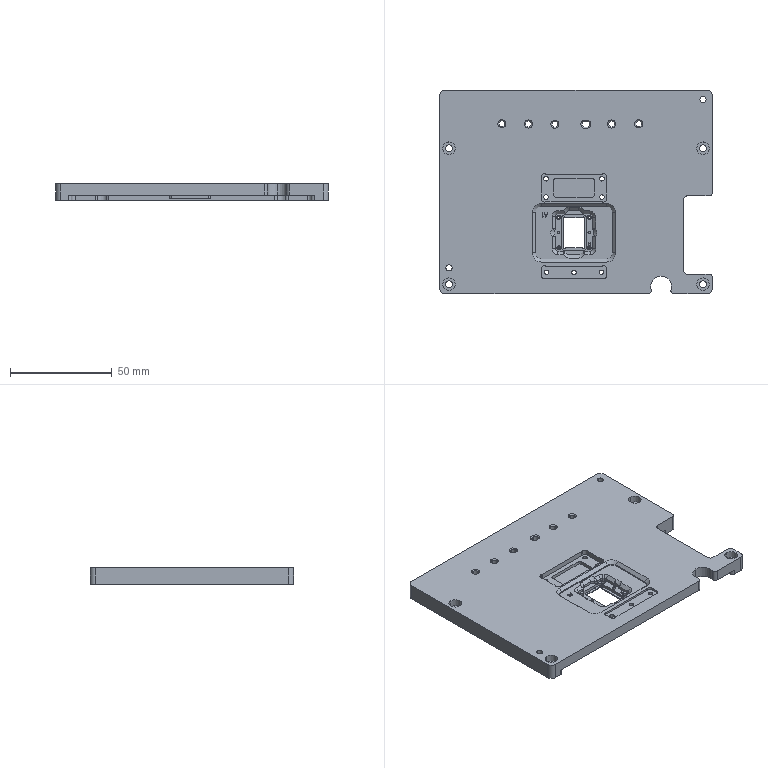NC program | NX | posted with a generic post | part box 134 x 100 x 8 mm
Lines 1537 to 2718 of 3418:
(ZLEVEL_PROFILE_COPY_COPY_COPY_1_COPY_COPY_1_COPY_COPY_COPY_1_COPY_COPY_1_COPY )
N3036 T20 M6
N3038 G54
N3040 G17 G0 G90 X2.531 Y-10.727 S9500 M3
N3042 G43 Z30. H20
N3044 Z0.1
N3046 G94 G1 X2.5 Y-10.6 Z0.093 F1000.
N3048 Y-8.627 Z-0.01
N3050 X2.387 Y-8.335 Z-0.027
N3052 X2.165 Y-8.113 Z-0.043
N3054 X1.873 Y-8. Z-0.06
N3056 X0.127 Z-0.151
N3058 X-0.165 Y-8.113 Z-0.167
N3060 X-0.387 Y-8.335 Z-0.184
N3062 X-0.5 Y-8.627 Z-0.2
N3064 Y-10.6 Z-0.304
N3066 X-0.629 Y-11.134 Z-0.333
N3068 X-0.898 Y-11.614 Z-0.361
N3070 X-1.286 Y-12.002 Z-0.39
N3072 X-1.766 Y-12.271 Z-0.419
N3074 X-2.3 Y-12.4 Z-0.448
N3076 X-4.337 Z-0.554
N3078 X-4.521 Y-12.501 Z-0.565
N3080 X-4.614 Y-12.649 Z-0.575
N3082 X-4.633 Y-12.814 Z-0.583
N3084 X-4.581 Y-12.971 Z-0.592
N3086 X-4.468 Y-13.093 Z-0.601
N3088 X-4.254 Y-13.176 Z-0.613
N3090 X-4.012 Y-13.366 Z-0.629
N3092 X-3.839 Y-13.62 Z-0.645
N3094 X-3.75 Y-13.914 Z-0.661
N3096 Y-20. Z-0.98
N3098 Y-25.944
N3100 G2 X-4.386 Y-26.876 R1.
N3102 G3 X-4.25 Y-27.6 R0.375
N3104 G1 X-2.5
N3106 G2 X-0.5 Y-29.6 R2.
N3108 G1 Y-31.25
N3110 G3 X0.25 Y-32. R0.75
N3112 G1 X1.75
N3114 G3 X2.5 Y-31.25 R0.75
N3116 G1 Y-29.6
N3118 G2 X4.5 Y-27.6 R2.
N3120 G1 X6.25
N3122 G3 X6.386 Y-26.876 R0.375
N3124 G2 X5.75 Y-25.944 R1.
N3126 G1 Y-14.056
N3128 G2 X6.386 Y-13.124 R1.
N3130 G3 X6.25 Y-12.4 R0.375
N3132 G1 X4.5
N3134 G2 X2.5 Y-10.4 R2.
N3136 G1 Y-8.75
N3138 G3 X1.75 Y-8. R0.75
N3140 G1 X0.25
N3142 G3 X-0.5 Y-8.75 R0.75
N3144 G1 Y-10.4
N3146 G2 X-2.5 Y-12.4 R2.
N3148 G1 X-4.25
N3150 G3 X-4.386 Y-13.124 R0.375
N3152 G2 X-3.75 Y-14.056 R1.
N3154 G1 Y-20.
N3156 Y-23.867 Z-1.048
N3158 Y-25.944
N3160 G2 X-4.386 Y-26.876 R1.
N3162 G3 X-4.25 Y-27.6 R0.375
N3164 G1 X-2.5
N3166 G2 X-0.5 Y-29.6 R2.
N3168 G1 Y-31.25
N3170 G3 X0.25 Y-32. R0.75
N3172 G1 X1.75
N3174 G3 X2.5 Y-31.25 R0.75
N3176 G1 Y-29.6
N3178 G2 X4.5 Y-27.6 R2.
N3180 G1 X6.25
N3182 G3 X6.386 Y-26.876 R0.375
N3184 G2 X5.75 Y-25.944 R1.
N3186 G1 Y-14.056
N3188 G2 X6.386 Y-13.124 R1.
N3190 G3 X6.25 Y-12.4 R0.375
N3192 G1 X4.5
N3194 G2 X2.5 Y-10.4 R2.
N3196 G1 Y-8.75
N3198 G3 X1.75 Y-8. R0.75
N3200 G1 X0.25
N3202 G3 X-0.5 Y-8.75 R0.75
N3204 G1 Y-10.4
N3206 G2 X-2.5 Y-12.4 R2.
N3208 G1 X-4.25
N3210 G3 X-4.386 Y-13.124 R0.375
N3212 G2 X-3.75 Y-14.056 R1.
N3214 G1 Y-20.
N3216 Y-23.867 Z-1.115
N3218 Y-25.944
N3220 G2 X-4.386 Y-26.876 R1.
N3222 G3 X-4.25 Y-27.6 R0.375
N3224 G1 X-2.5
N3226 G2 X-0.5 Y-29.6 R2.
N3228 G1 Y-31.25
N3230 G3 X0.25 Y-32. R0.75
N3232 G1 X1.75
N3234 G3 X2.5 Y-31.25 R0.75
N3236 G1 Y-29.6
N3238 G2 X4.5 Y-27.6 R2.
N3240 G1 X6.25
N3242 G3 X6.386 Y-26.876 R0.375
N3244 G2 X5.75 Y-25.944 R1.
N3246 G1 Y-14.056
N3248 G2 X6.386 Y-13.124 R1.
N3250 G3 X6.25 Y-12.4 R0.375
N3252 G1 X4.5
N3254 G2 X2.5 Y-10.4 R2.
N3256 G1 Y-8.75
N3258 G3 X1.75 Y-8. R0.75
N3260 G1 X0.25
N3262 G3 X-0.5 Y-8.75 R0.75
N3264 G1 Y-10.4
N3266 G2 X-2.5 Y-12.4 R2.
N3268 G1 X-4.25
N3270 G3 X-4.386 Y-13.124 R0.375
N3272 G2 X-3.75 Y-14.056 R1.
N3274 G1 Y-20.
N3276 Y-23.867 Z-1.183
N3278 Y-25.944
N3280 G2 X-4.386 Y-26.876 R1.
N3282 G3 X-4.25 Y-27.6 R0.375
N3284 G1 X-2.5
N3286 G2 X-0.5 Y-29.6 R2.
N3288 G1 Y-31.25
N3290 G3 X0.25 Y-32. R0.75
N3292 G1 X1.75
N3294 G3 X2.5 Y-31.25 R0.75
N3296 G1 Y-29.6
N3298 G2 X4.5 Y-27.6 R2.
N3300 G1 X6.25
N3302 G3 X6.386 Y-26.876 R0.375
N3304 G2 X5.75 Y-25.944 R1.
N3306 G1 Y-14.056
N3308 G2 X6.386 Y-13.124 R1.
N3310 G3 X6.25 Y-12.4 R0.375
N3312 G1 X4.5
N3314 G2 X2.5 Y-10.4 R2.
N3316 G1 Y-8.75
N3318 G3 X1.75 Y-8. R0.75
N3320 G1 X0.25
N3322 G3 X-0.5 Y-8.75 R0.75
N3324 G1 Y-10.4
N3326 G2 X-2.5 Y-12.4 R2.
N3328 G1 X-4.25
N3330 G3 X-4.386 Y-13.124 R0.375
N3332 G2 X-3.75 Y-14.056 R1.
N3334 G1 Y-20.
N3336 Y-23.867 Z-1.25
N3338 Y-25.944
N3340 G2 X-4.386 Y-26.876 R1.
N3342 G3 X-4.25 Y-27.6 R0.375
N3344 G1 X-2.5
N3346 G2 X-0.5 Y-29.6 R2.
N3348 G1 Y-31.25
N3350 G3 X0.25 Y-32. R0.75
N3352 G1 X1.75
N3354 G3 X2.5 Y-31.25 R0.75
N3356 G1 Y-29.6
N3358 G2 X4.5 Y-27.6 R2.
N3360 G1 X6.25
N3362 G3 X6.386 Y-26.876 R0.375
N3364 G2 X5.75 Y-25.944 R1.
N3366 G1 Y-14.056
N3368 G2 X6.386 Y-13.124 R1.
N3370 G3 X6.25 Y-12.4 R0.375
N3372 G1 X4.5
N3374 G2 X2.5 Y-10.4 R2.
N3376 G1 Y-8.75
N3378 G3 X1.75 Y-8. R0.75
N3380 G1 X0.25
N3382 G3 X-0.5 Y-8.75 R0.75
N3384 G1 Y-10.4
N3386 G2 X-2.5 Y-12.4 R2.
N3388 G1 X-4.25
N3390 G3 X-4.386 Y-13.124 R0.375
N3392 G2 X-3.75 Y-14.056 R1.
N3394 G1 Y-23.867
N3396 Z-0.25
N3398 G0 Z30.
(ZLEVEL_PROFILE_COPY_COPY_COPY_1_COPY_COPY_1_COPY_COPY_COPY_1_COPY_COPY_1_COPY_)
N3400 X0.084 Y-31.184
N3402 Z0.1
N3404 G1 X-0.086 Y-30.894 Z0.082
N3406 X-0.155 Y-30.482 Z0.06
N3408 X-0.073 Y-30.072 Z0.039
N3410 X0.076 Y-29.807 Z0.023
N3412 X0.292 Y-29.587 Z0.007
N3414 X0.559 Y-29.433 Z-0.01
N3416 X0.857 Y-29.354 Z-0.026
N3418 X1.161 Y-29.356 Z-0.042
N3420 X1.469 Y-29.445 Z-0.059
N3422 X1.742 Y-29.615 Z-0.075
N3424 X1.957 Y-29.853 Z-0.092
N3426 X2.092 Y-30.124 Z-0.108
N3428 X2.155 Y-30.524 Z-0.129
N3430 X2.075 Y-30.922 Z-0.151
N3432 X1.864 Y-31.267 Z-0.172
N3434 X1.546 Y-31.518 Z-0.193
N3436 X1.161 Y-31.644 Z-0.214
N3438 X1. Y-31.645 Z-0.223
N3440 X0.848 Z-0.231
N3442 X0.451 Y-31.516 Z-0.253
N3444 X0.125 Y-31.254 Z-0.274
N3446 X-0.086 Y-30.894 Z-0.296
N3448 X-0.155 Y-30.482 Z-0.318
N3450 X-0.073 Y-30.072 Z-0.34
N3452 X0.076 Y-29.807 Z-0.356
N3454 X0.292 Y-29.587 Z-0.372
N3456 X0.559 Y-29.433 Z-0.388
N3458 X0.857 Y-29.354 Z-0.405
N3460 X1.161 Y-29.356 Z-0.42
N3462 X1.469 Y-29.445 Z-0.437
N3464 X1.742 Y-29.615 Z-0.454
N3466 X1.957 Y-29.853 Z-0.471
N3468 X2.092 Y-30.124 Z-0.487
N3470 X2.155 Y-30.524 Z-0.508
N3472 X2.075 Y-30.922 Z-0.529
N3474 X1.864 Y-31.267 Z-0.55
N3476 X1.546 Y-31.518 Z-0.572
N3478 X1.161 Y-31.644 Z-0.593
N3480 X1. Y-31.645 Z-0.601
N3482 X0.848 Z-0.609
N3484 X0.451 Y-31.516 Z-0.631
N3486 X0.125 Y-31.254 Z-0.653
N3488 X-0.086 Y-30.894 Z-0.675
N3490 X-0.155 Y-30.482 Z-0.697
N3492 X-0.073 Y-30.072 Z-0.719
N3494 X0.076 Y-29.807 Z-0.735
N3496 X0.292 Y-29.587 Z-0.751
N3498 X0.559 Y-29.433 Z-0.767
N3500 X0.857 Y-29.354 Z-0.783
N3502 X1.161 Y-29.356 Z-0.799
N3504 X1.469 Y-29.445 Z-0.816
N3506 X1.742 Y-29.615 Z-0.833
N3508 X1.957 Y-29.853 Z-0.85
N3510 X2.092 Y-30.124 Z-0.865
N3512 X2.155 Y-30.524 Z-0.887
N3514 X2.075 Y-30.922 Z-0.908
N3516 X1.864 Y-31.267 Z-0.929
N3518 X1.546 Y-31.518 Z-0.95
N3520 X1.161 Y-31.644 Z-0.972
N3522 X1. Y-31.645 Z-0.98
N3524 G2 X-0.145 Y-30.5 R1.145
N3526 X1. Y-31.645 R-1.145
N3528 G1 X0.928 Y-31.643 Z-0.981
N3530 X0.857 Y-31.636 Z-0.983
N3532 X0.786 Y-31.625 Z-0.984
N3534 X0.717 Y-31.609 Z-0.985
N3536 X0.648 Y-31.589 Z-0.986
N3538 X0.58 Y-31.565 Z-0.988
N3540 X0.515 Y-31.537 Z-0.989
N3542 X0.451 Y-31.505 Z-0.99
N3544 X0.389 Y-31.468 Z-0.991
N3546 X0.33 Y-31.428 Z-0.993
N3548 X0.273 Y-31.385 Z-0.994
N3550 X0.219 Y-31.337 Z-0.995
N3552 X0.168 Y-31.287 Z-0.996
N3554 X0.121 Y-31.233 Z-0.998
N3556 X0.077 Y-31.177 Z-0.999
N3558 X0.036 Y-31.118 Z-1.
N3560 X-0.001 Y-31.057 Z-1.001
N3562 X-0.033 Y-30.993 Z-1.003
N3564 X-0.062 Y-30.927 Z-1.004
N3566 X-0.087 Y-30.86 Z-1.005
N3568 X-0.107 Y-30.791 Z-1.006
N3570 X-0.123 Y-30.722 Z-1.008
N3572 X-0.135 Y-30.651 Z-1.009
N3574 X-0.142 Y-30.58 Z-1.01
N3576 X-0.145 Y-30.508 Z-1.011
N3578 X-0.143 Y-30.437 Z-1.013
N3580 X-0.137 Y-30.365 Z-1.014
N3582 X-0.126 Y-30.295 Z-1.015
N3584 X-0.111 Y-30.225 Z-1.016
N3586 X-0.092 Y-30.156 Z-1.018
N3588 X-0.068 Y-30.088 Z-1.019
N3590 X-0.04 Y-30.022 Z-1.02
N3592 X-0.009 Y-29.958 Z-1.021
N3594 X0.027 Y-29.896 Z-1.023
N3596 X0.067 Y-29.836 Z-1.024
N3598 X0.11 Y-29.779 Z-1.025
N3600 X0.157 Y-29.725 Z-1.026
N3602 X0.207 Y-29.674 Z-1.028
N3604 X0.26 Y-29.626 Z-1.029
N3606 X0.316 Y-29.581 Z-1.03
N3608 X0.375 Y-29.541 Z-1.031
N3610 X0.436 Y-29.503 Z-1.033
N3612 X0.5 Y-29.47 Z-1.034
N3614 X0.565 Y-29.441 Z-1.035
N3616 X0.632 Y-29.416 Z-1.036
N3618 X0.701 Y-29.395 Z-1.038
N3620 X0.77 Y-29.378 Z-1.039
N3622 X0.841 Y-29.366 Z-1.04
N3624 X0.912 Y-29.358 Z-1.041
N3626 X0.984 Y-29.355 Z-1.043
N3628 X1.055 Y-29.356 Z-1.044
N3630 X1.126 Y-29.362 Z-1.045
N3632 X1.197 Y-29.372 Z-1.046
N3634 X1.267 Y-29.387 Z-1.048
N3636 X1.337 Y-29.406 Z-1.049
N3638 X1.404 Y-29.429 Z-1.05
N3640 X1.47 Y-29.456 Z-1.051
N3642 X1.535 Y-29.488 Z-1.053
N3644 X1.597 Y-29.523 Z-1.054
N3646 X1.657 Y-29.562 Z-1.055
N3648 X1.714 Y-29.605 Z-1.056
N3650 X1.769 Y-29.651 Z-1.058
N3652 X1.82 Y-29.701 Z-1.059
N3654 X1.869 Y-29.754 Z-1.06
N3656 G2 X1. Y-31.645 R1.145
N3658 G1 X0.928 Y-31.643 Z-1.061
N3660 X0.857 Y-31.636 Z-1.063
N3662 X0.786 Y-31.625 Z-1.064
N3664 X0.717 Y-31.609 Z-1.065
N3666 X0.648 Y-31.589 Z-1.066
N3668 X0.58 Y-31.565 Z-1.068
N3670 X0.515 Y-31.537 Z-1.069
N3672 X0.451 Y-31.505 Z-1.07
N3674 X0.389 Y-31.468 Z-1.071
N3676 X0.33 Y-31.428 Z-1.073
N3678 X0.273 Y-31.385 Z-1.074
N3680 X0.219 Y-31.337 Z-1.075
N3682 X0.168 Y-31.287 Z-1.076
N3684 X0.121 Y-31.233 Z-1.078
N3686 X0.077 Y-31.177 Z-1.079
N3688 X0.036 Y-31.118 Z-1.08
N3690 X-0.001 Y-31.057 Z-1.081
N3692 X-0.034 Y-30.993 Z-1.083
N3694 X-0.062 Y-30.927 Z-1.084
N3696 X-0.087 Y-30.86 Z-1.085
N3698 X-0.107 Y-30.791 Z-1.086
N3700 X-0.123 Y-30.722 Z-1.088
N3702 X-0.135 Y-30.651 Z-1.089
N3704 X-0.142 Y-30.58 Z-1.09
N3706 X-0.145 Y-30.508 Z-1.091
N3708 X-0.143 Y-30.437 Z-1.093
N3710 X-0.137 Y-30.365 Z-1.094
N3712 X-0.126 Y-30.295 Z-1.095
N3714 X-0.111 Y-30.225 Z-1.096
N3716 X-0.092 Y-30.156 Z-1.098
N3718 X-0.068 Y-30.088 Z-1.099
N3720 X-0.04 Y-30.022 Z-1.1
N3722 X-0.009 Y-29.958 Z-1.101
N3724 X0.027 Y-29.896 Z-1.103
N3726 X0.067 Y-29.836 Z-1.104
N3728 X0.11 Y-29.779 Z-1.105
N3730 X0.157 Y-29.725 Z-1.106
N3732 X0.207 Y-29.674 Z-1.108
N3734 X0.26 Y-29.626 Z-1.109
N3736 X0.316 Y-29.581 Z-1.11
N3738 X0.375 Y-29.541 Z-1.111
N3740 X0.436 Y-29.503 Z-1.113
N3742 X0.5 Y-29.47 Z-1.114
N3744 X0.565 Y-29.441 Z-1.115
N3746 X0.632 Y-29.416 Z-1.116
N3748 X0.701 Y-29.395 Z-1.118
N3750 X0.77 Y-29.378 Z-1.119
N3752 X0.841 Y-29.366 Z-1.12
N3754 X0.912 Y-29.358 Z-1.121
N3756 X0.984 Y-29.355 Z-1.123
N3758 X1.055 Y-29.356 Z-1.124
N3760 X1.126 Y-29.362 Z-1.125
N3762 X1.197 Y-29.372 Z-1.126
N3764 X1.268 Y-29.386 Z-1.128
N3766 X1.337 Y-29.406 Z-1.129
N3768 X1.404 Y-29.429 Z-1.13
N3770 X1.47 Y-29.456 Z-1.131
N3772 X1.535 Y-29.488 Z-1.133
N3774 G2 X1. Y-31.645 R1.145
N3776 G1 X0.928 Y-31.643 Z-1.134
N3778 X0.857 Y-31.636 Z-1.135
N3780 X0.786 Y-31.625 Z-1.136
N3782 X0.717 Y-31.609 Z-1.138
N3784 X0.648 Y-31.589 Z-1.139
N3786 X0.58 Y-31.565 Z-1.14
N3788 X0.515 Y-31.537 Z-1.141
N3790 X0.451 Y-31.505 Z-1.143
N3792 X0.389 Y-31.468 Z-1.144
N3794 X0.33 Y-31.428 Z-1.145
N3796 X0.273 Y-31.385 Z-1.146
N3798 X0.219 Y-31.337 Z-1.148
N3800 X0.168 Y-31.287 Z-1.149
N3802 X0.121 Y-31.233 Z-1.15
N3804 X0.077 Y-31.177 Z-1.151
N3806 X0.036 Y-31.118 Z-1.153
N3808 X-0.001 Y-31.057 Z-1.154
N3810 X-0.033 Y-30.993 Z-1.155
N3812 X-0.062 Y-30.927 Z-1.156
N3814 X-0.087 Y-30.86 Z-1.158
N3816 X-0.107 Y-30.791 Z-1.159
N3818 X-0.123 Y-30.722 Z-1.16
N3820 X-0.135 Y-30.651 Z-1.161
N3822 X-0.142 Y-30.58 Z-1.163
N3824 X-0.145 Y-30.508 Z-1.164
N3826 X-0.143 Y-30.437 Z-1.165
N3828 X-0.137 Y-30.365 Z-1.166
N3830 X-0.126 Y-30.295 Z-1.168
N3832 X-0.111 Y-30.225 Z-1.169
N3834 X-0.092 Y-30.156 Z-1.17
N3836 X-0.068 Y-30.088 Z-1.171
N3838 X-0.04 Y-30.022 Z-1.173
N3840 X-0.009 Y-29.958 Z-1.174
N3842 X0.027 Y-29.896 Z-1.175
N3844 X0.067 Y-29.836 Z-1.176
N3846 X0.11 Y-29.779 Z-1.178
N3848 X0.157 Y-29.725 Z-1.179
N3850 X0.207 Y-29.674 Z-1.18
N3852 X0.26 Y-29.626 Z-1.181
N3854 X0.316 Y-29.581 Z-1.183
N3856 X0.375 Y-29.541 Z-1.184
N3858 X0.436 Y-29.503 Z-1.185
N3860 X0.5 Y-29.47 Z-1.186
N3862 X0.565 Y-29.441 Z-1.188
N3864 X0.632 Y-29.416 Z-1.189
N3866 X0.7 Y-29.395 Z-1.19
N3868 X0.77 Y-29.378 Z-1.191
N3870 X0.841 Y-29.366 Z-1.193
N3872 X0.912 Y-29.358 Z-1.194
N3874 X0.984 Y-29.355 Z-1.195
N3876 X1.055 Y-29.356 Z-1.196
N3878 X1.126 Y-29.362 Z-1.198
N3880 X1.197 Y-29.372 Z-1.199
N3882 X1.267 Y-29.387 Z-1.2
N3884 X1.337 Y-29.406 Z-1.201
N3886 X1.404 Y-29.428 Z-1.203
N3888 X1.47 Y-29.456 Z-1.204
N3890 X1.535 Y-29.488 Z-1.205
N3892 G2 X1. Y-31.645 R1.145
N3894 G1 X0.928 Y-31.643 Z-1.206
N3896 X0.857 Y-31.636 Z-1.208
N3898 X0.786 Y-31.625 Z-1.209
N3900 X0.717 Y-31.609 Z-1.21
N3902 X0.648 Y-31.589 Z-1.211
N3904 X0.58 Y-31.565 Z-1.213
N3906 X0.515 Y-31.537 Z-1.214
N3908 X0.451 Y-31.505 Z-1.215
N3910 X0.389 Y-31.468 Z-1.216
N3912 X0.329 Y-31.429 Z-1.218
N3914 X0.273 Y-31.385 Z-1.219
N3916 X0.219 Y-31.337 Z-1.22
N3918 X0.168 Y-31.287 Z-1.221
N3920 X0.121 Y-31.233 Z-1.223
N3922 X0.077 Y-31.177 Z-1.224
N3924 X0.036 Y-31.118 Z-1.225
N3926 X-0.001 Y-31.057 Z-1.226
N3928 X-0.033 Y-30.993 Z-1.228
N3930 X-0.062 Y-30.927 Z-1.229
N3932 X-0.087 Y-30.86 Z-1.23
N3934 X-0.107 Y-30.791 Z-1.231
N3936 X-0.123 Y-30.722 Z-1.233
N3938 X-0.135 Y-30.651 Z-1.234
N3940 X-0.142 Y-30.58 Z-1.235
N3942 X-0.145 Y-30.508 Z-1.236
N3944 X-0.143 Y-30.437 Z-1.238
N3946 X-0.137 Y-30.365 Z-1.239
N3948 X-0.126 Y-30.295 Z-1.24
N3950 X-0.111 Y-30.225 Z-1.241
N3952 X-0.092 Y-30.156 Z-1.243
N3954 X-0.068 Y-30.088 Z-1.244
N3956 X-0.04 Y-30.022 Z-1.245
N3958 X-0.009 Y-29.958 Z-1.246
N3960 X0.027 Y-29.896 Z-1.248
N3962 X0.067 Y-29.836 Z-1.249
N3964 X0.11 Y-29.779 Z-1.25
N3966 X0.157 Y-29.725 Z-1.251
N3968 X0.207 Y-29.674 Z-1.253
N3970 X0.26 Y-29.626 Z-1.254
N3972 X0.316 Y-29.581 Z-1.255
N3974 X0.375 Y-29.541 Z-1.256
N3976 X0.436 Y-29.503 Z-1.258
N3978 X0.5 Y-29.47 Z-1.259
N3980 X0.565 Y-29.441 Z-1.26
N3982 X0.632 Y-29.416 Z-1.261
N3984 X0.7 Y-29.394 Z-1.263
N3986 X0.77 Y-29.378 Z-1.264
N3988 X0.841 Y-29.366 Z-1.265
N3990 X0.912 Y-29.358 Z-1.266
N3992 X0.984 Y-29.355 Z-1.268
N3994 X1.055 Y-29.356 Z-1.269
N3996 X1.126 Y-29.362 Z-1.27
N3998 X1.197 Y-29.372 Z-1.271
N4000 X1.267 Y-29.387 Z-1.273
N4002 X1.337 Y-29.406 Z-1.274
N4004 X1.404 Y-29.428 Z-1.275
N4006 X1.47 Y-29.456 Z-1.276
N4008 X1.535 Y-29.488 Z-1.278
N4010 G2 X1. Y-31.645 R1.145
N4012 G1 X0.928 Y-31.643 Z-1.279
N4014 X0.857 Y-31.636 Z-1.28
N4016 X0.786 Y-31.625 Z-1.281
N4018 X0.717 Y-31.609 Z-1.283
N4020 X0.648 Y-31.589 Z-1.284
N4022 X0.58 Y-31.566 Z-1.285
N4024 X0.515 Y-31.537 Z-1.286
N4026 X0.451 Y-31.505 Z-1.288
N4028 X0.389 Y-31.468 Z-1.289
N4030 X0.33 Y-31.428 Z-1.29
N4032 X0.273 Y-31.385 Z-1.291
N4034 X0.219 Y-31.337 Z-1.293
N4036 X0.168 Y-31.287 Z-1.294
N4038 X0.121 Y-31.233 Z-1.295
N4040 X0.077 Y-31.177 Z-1.296
N4042 X0.036 Y-31.118 Z-1.298
N4044 X-0.001 Y-31.057 Z-1.299
N4046 X-0.034 Y-30.993 Z-1.3
N4048 X-0.062 Y-30.927 Z-1.301
N4050 X-0.087 Y-30.86 Z-1.303
N4052 X-0.107 Y-30.791 Z-1.304
N4054 X-0.123 Y-30.722 Z-1.305
N4056 X-0.135 Y-30.651 Z-1.306
N4058 X-0.142 Y-30.58 Z-1.308
N4060 X-0.145 Y-30.508 Z-1.309
N4062 X-0.143 Y-30.437 Z-1.31
N4064 X-0.137 Y-30.365 Z-1.311
N4066 X-0.126 Y-30.295 Z-1.313
N4068 X-0.111 Y-30.225 Z-1.314
N4070 X-0.092 Y-30.156 Z-1.315
N4072 X-0.068 Y-30.088 Z-1.316
N4074 X-0.04 Y-30.022 Z-1.318
N4076 X-0.009 Y-29.958 Z-1.319
N4078 X0.027 Y-29.896 Z-1.32
N4080 X0.067 Y-29.836 Z-1.321
N4082 X0.11 Y-29.779 Z-1.323
N4084 X0.157 Y-29.725 Z-1.324
N4086 X0.207 Y-29.674 Z-1.325
N4088 X0.26 Y-29.626 Z-1.326
N4090 X0.316 Y-29.581 Z-1.328
N4092 X0.375 Y-29.541 Z-1.329
N4094 X0.436 Y-29.503 Z-1.33
N4096 X0.5 Y-29.47 Z-1.331
N4098 X0.565 Y-29.441 Z-1.333
N4100 X0.632 Y-29.416 Z-1.334
N4102 X0.701 Y-29.395 Z-1.335
N4104 X0.77 Y-29.378 Z-1.336
N4106 X0.841 Y-29.366 Z-1.338
N4108 X0.912 Y-29.358 Z-1.339
N4110 X0.984 Y-29.355 Z-1.34
N4112 X1.055 Y-29.356 Z-1.341
N4114 X1.127 Y-29.361 Z-1.343
N4116 X1.197 Y-29.372 Z-1.344
N4118 X1.268 Y-29.386 Z-1.345
N4120 X1.337 Y-29.406 Z-1.346
N4122 X1.404 Y-29.428 Z-1.348
N4124 X1.47 Y-29.456 Z-1.349
N4126 X1.535 Y-29.488 Z-1.35
N4128 G2 X2.012 Y-31.035 R1.145
N4130 X1.535 Y-29.488 R-1.145
N4132 G1 Z-0.35
N4134 G0 Z30.
N4136 X0.084 Y-10.184
N4138 Z0.1
N4140 G1 X-0.086 Y-9.894 Z0.082
N4142 X-0.155 Y-9.482 Z0.06
N4144 X-0.073 Y-9.072 Z0.039
N4146 X0.076 Y-8.807 Z0.023
N4148 X0.292 Y-8.587 Z0.007
N4150 X0.559 Y-8.433 Z-0.01
N4152 X0.857 Y-8.354 Z-0.026
N4154 X1.161 Y-8.356 Z-0.042
N4156 X1.469 Y-8.445 Z-0.059
N4158 X1.742 Y-8.615 Z-0.075
N4160 X1.957 Y-8.853 Z-0.092
N4162 X2.092 Y-9.124 Z-0.108
N4164 X2.155 Y-9.524 Z-0.129
N4166 X2.075 Y-9.922 Z-0.151
N4168 X1.864 Y-10.267 Z-0.172
N4170 X1.546 Y-10.518 Z-0.193
N4172 X1.161 Y-10.644 Z-0.214
N4174 X1. Y-10.645 Z-0.223
N4176 X0.848 Z-0.231
N4178 X0.451 Y-10.516 Z-0.253
N4180 X0.125 Y-10.254 Z-0.274
N4182 X-0.086 Y-9.894 Z-0.296
N4184 X-0.155 Y-9.482 Z-0.318
N4186 X-0.073 Y-9.072 Z-0.34
N4188 X0.076 Y-8.807 Z-0.356
N4190 X0.292 Y-8.587 Z-0.372
N4192 X0.559 Y-8.433 Z-0.388
N4194 X0.857 Y-8.354 Z-0.405
N4196 X1.161 Y-8.356 Z-0.42
N4198 X1.469 Y-8.445 Z-0.437
N4200 X1.742 Y-8.615 Z-0.454
N4202 X1.957 Y-8.853 Z-0.471
N4204 X2.092 Y-9.124 Z-0.487
N4206 X2.155 Y-9.524 Z-0.508
N4208 X2.075 Y-9.922 Z-0.529
N4210 X1.864 Y-10.267 Z-0.55
N4212 X1.546 Y-10.518 Z-0.572
N4214 X1.161 Y-10.644 Z-0.593
N4216 X1. Y-10.645 Z-0.601
N4218 X0.848 Z-0.609
N4220 X0.451 Y-10.516 Z-0.631
N4222 X0.125 Y-10.254 Z-0.653
N4224 X-0.086 Y-9.894 Z-0.675
N4226 X-0.155 Y-9.482 Z-0.697
N4228 X-0.073 Y-9.072 Z-0.719
N4230 X0.076 Y-8.807 Z-0.735
N4232 X0.292 Y-8.587 Z-0.751
N4234 X0.559 Y-8.433 Z-0.767
N4236 X0.857 Y-8.354 Z-0.783
N4238 X1.161 Y-8.356 Z-0.799
N4240 X1.469 Y-8.445 Z-0.816
N4242 X1.742 Y-8.615 Z-0.833
N4244 X1.957 Y-8.853 Z-0.85
N4246 X2.092 Y-9.124 Z-0.865
N4248 X2.155 Y-9.524 Z-0.887
N4250 X2.075 Y-9.922 Z-0.908
N4252 X1.864 Y-10.267 Z-0.929
N4254 X1.546 Y-10.518 Z-0.95
N4256 X1.161 Y-10.644 Z-0.972
N4258 X1. Y-10.645 Z-0.98
N4260 G2 X-0.145 Y-9.5 R1.145
N4262 X1. Y-10.645 R-1.145
N4264 G1 X0.928 Y-10.643 Z-0.981
N4266 X0.857 Y-10.636 Z-0.983
N4268 X0.786 Y-10.625 Z-0.984
N4270 X0.717 Y-10.609 Z-0.985
N4272 X0.648 Y-10.589 Z-0.986
N4274 X0.58 Y-10.565 Z-0.988
N4276 X0.515 Y-10.537 Z-0.989
N4278 X0.451 Y-10.505 Z-0.99
N4280 X0.389 Y-10.468 Z-0.991
N4282 X0.33 Y-10.428 Z-0.993
N4284 X0.273 Y-10.385 Z-0.994
N4286 X0.219 Y-10.337 Z-0.995
N4288 X0.168 Y-10.287 Z-0.996
N4290 X0.121 Y-10.233 Z-0.998
N4292 X0.077 Y-10.177 Z-0.999
N4294 X0.036 Y-10.118 Z-1.
N4296 X-0.001 Y-10.057 Z-1.001
N4298 X-0.033 Y-9.993 Z-1.003
N4300 X-0.062 Y-9.927 Z-1.004
N4302 X-0.087 Y-9.86 Z-1.005
N4304 X-0.107 Y-9.791 Z-1.006
N4306 X-0.123 Y-9.722 Z-1.008
N4308 X-0.135 Y-9.651 Z-1.009
N4310 X-0.142 Y-9.58 Z-1.01
N4312 X-0.145 Y-9.508 Z-1.011
N4314 X-0.143 Y-9.437 Z-1.013
N4316 X-0.137 Y-9.365 Z-1.014
N4318 X-0.127 Y-9.295 Z-1.015
N4320 X-0.111 Y-9.225 Z-1.016
N4322 X-0.092 Y-9.156 Z-1.018
N4324 X-0.068 Y-9.088 Z-1.019
N4326 X-0.04 Y-9.022 Z-1.02
N4328 X-0.009 Y-8.958 Z-1.021
N4330 X0.027 Y-8.896 Z-1.023
N4332 X0.067 Y-8.836 Z-1.024
N4334 X0.11 Y-8.779 Z-1.025
N4336 X0.157 Y-8.725 Z-1.026
N4338 X0.207 Y-8.674 Z-1.028
N4340 X0.26 Y-8.626 Z-1.029
N4342 X0.316 Y-8.581 Z-1.03
N4344 X0.375 Y-8.541 Z-1.031
N4346 X0.436 Y-8.503 Z-1.033
N4348 X0.5 Y-8.47 Z-1.034
N4350 X0.565 Y-8.441 Z-1.035
N4352 X0.632 Y-8.416 Z-1.036
N4354 X0.701 Y-8.395 Z-1.038
N4356 X0.77 Y-8.378 Z-1.039
N4358 X0.841 Y-8.366 Z-1.04
N4360 X0.912 Y-8.358 Z-1.041
N4362 X0.984 Y-8.355 Z-1.043
N4364 X1.055 Y-8.356 Z-1.044
N4366 X1.126 Y-8.362 Z-1.045
N4368 X1.197 Y-8.372 Z-1.046
N4370 X1.267 Y-8.387 Z-1.048
N4372 X1.337 Y-8.406 Z-1.049
N4374 X1.404 Y-8.429 Z-1.05
N4376 X1.47 Y-8.456 Z-1.051
N4378 X1.535 Y-8.488 Z-1.053
N4380 X1.597 Y-8.523 Z-1.054
N4382 X1.657 Y-8.562 Z-1.055
N4384 X1.714 Y-8.605 Z-1.056
N4386 X1.769 Y-8.651 Z-1.058
N4388 X1.82 Y-8.701 Z-1.059
N4390 X1.869 Y-8.754 Z-1.06
N4392 G2 X1. Y-10.645 R1.145
N4394 G1 X0.928 Y-10.643 Z-1.061
N4396 X0.857 Y-10.636 Z-1.063
N4398 X0.786 Y-10.625 Z-1.064
N4400 X0.717 Y-10.609 Z-1.065
N4402 X0.648 Y-10.589 Z-1.066
N4404 X0.58 Y-10.565 Z-1.068
N4406 X0.515 Y-10.537 Z-1.069
N4408 X0.451 Y-10.505 Z-1.07
N4410 X0.389 Y-10.468 Z-1.071
N4412 X0.33 Y-10.428 Z-1.073
N4414 X0.273 Y-10.385 Z-1.074
N4416 X0.219 Y-10.337 Z-1.075
N4418 X0.168 Y-10.287 Z-1.076
N4420 X0.121 Y-10.233 Z-1.078
N4422 X0.077 Y-10.177 Z-1.079
N4424 X0.036 Y-10.118 Z-1.08
N4426 X-0.001 Y-10.057 Z-1.081
N4428 X-0.034 Y-9.993 Z-1.083
N4430 X-0.062 Y-9.927 Z-1.084
N4432 X-0.087 Y-9.86 Z-1.085
N4434 X-0.107 Y-9.791 Z-1.086
N4436 X-0.124 Y-9.722 Z-1.088
N4438 X-0.135 Y-9.651 Z-1.089
N4440 X-0.142 Y-9.58 Z-1.09
N4442 X-0.145 Y-9.508 Z-1.091
N4444 X-0.143 Y-9.437 Z-1.093
N4446 X-0.137 Y-9.365 Z-1.094
N4448 X-0.126 Y-9.295 Z-1.095
N4450 X-0.111 Y-9.225 Z-1.096
N4452 X-0.092 Y-9.156 Z-1.098
N4454 X-0.068 Y-9.088 Z-1.099
N4456 X-0.04 Y-9.022 Z-1.1
N4458 X-0.009 Y-8.958 Z-1.101
N4460 X0.027 Y-8.896 Z-1.103
N4462 X0.067 Y-8.836 Z-1.104
N4464 X0.11 Y-8.779 Z-1.105
N4466 X0.157 Y-8.725 Z-1.106
N4468 X0.207 Y-8.674 Z-1.108
N4470 X0.26 Y-8.626 Z-1.109
N4472 X0.316 Y-8.581 Z-1.11
N4474 X0.375 Y-8.541 Z-1.111
N4476 X0.436 Y-8.503 Z-1.113
N4478 X0.5 Y-8.47 Z-1.114
N4480 X0.565 Y-8.441 Z-1.115
N4482 X0.632 Y-8.416 Z-1.116
N4484 X0.701 Y-8.395 Z-1.118
N4486 X0.77 Y-8.378 Z-1.119
N4488 X0.841 Y-8.366 Z-1.12
N4490 X0.912 Y-8.358 Z-1.121
N4492 X0.984 Y-8.355 Z-1.123
N4494 X1.055 Y-8.356 Z-1.124
N4496 X1.126 Y-8.362 Z-1.125
N4498 X1.197 Y-8.372 Z-1.126
N4500 X1.267 Y-8.387 Z-1.128
N4502 X1.337 Y-8.406 Z-1.129
N4504 X1.404 Y-8.429 Z-1.13
N4506 X1.47 Y-8.456 Z-1.131
N4508 X1.535 Y-8.488 Z-1.133
N4510 G2 X1. Y-10.645 R1.145
N4512 G1 X0.928 Y-10.643 Z-1.134
N4514 X0.857 Y-10.636 Z-1.135
N4516 X0.786 Y-10.625 Z-1.136
N4518 X0.716 Y-10.61 Z-1.138
N4520 X0.648 Y-10.589 Z-1.139
N4522 X0.58 Y-10.566 Z-1.14
N4524 X0.515 Y-10.537 Z-1.141
N4526 X0.451 Y-10.505 Z-1.143
N4528 X0.389 Y-10.468 Z-1.144
N4530 X0.33 Y-10.428 Z-1.145
N4532 X0.273 Y-10.385 Z-1.146
N4534 X0.219 Y-10.338 Z-1.148
N4536 X0.168 Y-10.287 Z-1.149
N4538 X0.121 Y-10.233 Z-1.15
N4540 X0.077 Y-10.177 Z-1.151
N4542 X0.036 Y-10.118 Z-1.153
N4544 X-0.001 Y-10.057 Z-1.154
N4546 X-0.033 Y-9.993 Z-1.155
N4548 X-0.062 Y-9.927 Z-1.156
N4550 X-0.087 Y-9.86 Z-1.158
N4552 X-0.107 Y-9.791 Z-1.159
N4554 X-0.124 Y-9.722 Z-1.16
N4556 X-0.135 Y-9.651 Z-1.161
N4558 X-0.143 Y-9.58 Z-1.163
N4560 X-0.145 Y-9.508 Z-1.164
N4562 X-0.144 Y-9.437 Z-1.165
N4564 X-0.137 Y-9.365 Z-1.166
N4566 X-0.126 Y-9.295 Z-1.168
N4568 X-0.111 Y-9.225 Z-1.169
N4570 X-0.092 Y-9.156 Z-1.17
N4572 X-0.068 Y-9.088 Z-1.171
N4574 X-0.04 Y-9.022 Z-1.173
N4576 X-0.009 Y-8.958 Z-1.174
N4578 X0.027 Y-8.896 Z-1.175
N4580 X0.067 Y-8.836 Z-1.176
N4582 X0.11 Y-8.779 Z-1.178
N4584 X0.157 Y-8.725 Z-1.179
N4586 X0.207 Y-8.674 Z-1.18
N4588 X0.26 Y-8.626 Z-1.181
N4590 X0.316 Y-8.581 Z-1.183
N4592 X0.375 Y-8.541 Z-1.184
N4594 X0.436 Y-8.503 Z-1.185
N4596 X0.5 Y-8.47 Z-1.186
N4598 X0.565 Y-8.441 Z-1.188
N4600 X0.632 Y-8.416 Z-1.189
N4602 X0.7 Y-8.395 Z-1.19
N4604 X0.77 Y-8.378 Z-1.191
N4606 X0.841 Y-8.366 Z-1.193
N4608 X0.912 Y-8.358 Z-1.194
N4610 X0.984 Y-8.355 Z-1.195
N4612 X1.055 Y-8.356 Z-1.196
N4614 X1.126 Y-8.362 Z-1.198
N4616 X1.197 Y-8.372 Z-1.199
N4618 X1.267 Y-8.387 Z-1.2
N4620 X1.337 Y-8.406 Z-1.201
N4622 X1.404 Y-8.429 Z-1.203
N4624 X1.47 Y-8.456 Z-1.204
N4626 X1.535 Y-8.488 Z-1.205
N4628 G2 X1. Y-10.645 R1.145
N4630 G1 X0.928 Y-10.643 Z-1.206
N4632 X0.857 Y-10.636 Z-1.208
N4634 X0.786 Y-10.625 Z-1.209
N4636 X0.716 Y-10.61 Z-1.21
N4638 X0.648 Y-10.589 Z-1.211
N4640 X0.58 Y-10.566 Z-1.213
N4642 X0.515 Y-10.537 Z-1.214
N4644 X0.451 Y-10.505 Z-1.215
N4646 X0.389 Y-10.468 Z-1.216
N4648 X0.33 Y-10.428 Z-1.218
N4650 X0.273 Y-10.385 Z-1.219
N4652 X0.219 Y-10.338 Z-1.22
N4654 X0.168 Y-10.287 Z-1.221
N4656 X0.121 Y-10.233 Z-1.223
N4658 X0.077 Y-10.177 Z-1.224
N4660 X0.036 Y-10.118 Z-1.225
N4662 X-0.001 Y-10.057 Z-1.226
N4664 X-0.033 Y-9.993 Z-1.228
N4666 X-0.062 Y-9.927 Z-1.229
N4668 X-0.087 Y-9.86 Z-1.23
N4670 X-0.107 Y-9.791 Z-1.231
N4672 X-0.124 Y-9.722 Z-1.233
N4674 X-0.135 Y-9.651 Z-1.234
N4676 X-0.143 Y-9.58 Z-1.235
N4678 X-0.145 Y-9.508 Z-1.236
N4680 X-0.144 Y-9.437 Z-1.238
N4682 X-0.137 Y-9.365 Z-1.239
N4684 X-0.126 Y-9.295 Z-1.24
N4686 X-0.111 Y-9.225 Z-1.241
N4688 X-0.092 Y-9.156 Z-1.243
N4690 X-0.068 Y-9.088 Z-1.244
N4692 X-0.04 Y-9.022 Z-1.245
N4694 X-0.009 Y-8.958 Z-1.246
N4696 X0.027 Y-8.896 Z-1.248
N4698 X0.067 Y-8.836 Z-1.249
N4700 X0.11 Y-8.779 Z-1.25
N4702 X0.157 Y-8.725 Z-1.251
N4704 X0.207 Y-8.674 Z-1.253
N4706 X0.26 Y-8.626 Z-1.254
N4708 X0.316 Y-8.581 Z-1.255
N4710 X0.375 Y-8.541 Z-1.256
N4712 X0.436 Y-8.503 Z-1.258
N4714 X0.5 Y-8.47 Z-1.259
N4716 X0.565 Y-8.441 Z-1.26
N4718 X0.632 Y-8.416 Z-1.261
N4720 X0.7 Y-8.394 Z-1.263
N4722 X0.77 Y-8.378 Z-1.264
N4724 X0.841 Y-8.366 Z-1.265
N4726 X0.912 Y-8.358 Z-1.266
N4728 X0.984 Y-8.355 Z-1.268
N4730 X1.055 Y-8.356 Z-1.269
N4732 X1.126 Y-8.362 Z-1.27
N4734 X1.197 Y-8.372 Z-1.271
N4736 X1.267 Y-8.387 Z-1.273
N4738 X1.337 Y-8.406 Z-1.274
N4740 X1.404 Y-8.429 Z-1.275
N4742 X1.47 Y-8.456 Z-1.276
N4744 X1.535 Y-8.488 Z-1.278
N4746 G2 X1. Y-10.645 R1.145
N4748 G1 X0.928 Y-10.643 Z-1.279
N4750 X0.857 Y-10.636 Z-1.28
N4752 X0.786 Y-10.625 Z-1.281
N4754 X0.717 Y-10.609 Z-1.283
N4756 X0.648 Y-10.589 Z-1.284
N4758 X0.58 Y-10.566 Z-1.285
N4760 X0.515 Y-10.537 Z-1.286
N4762 X0.451 Y-10.505 Z-1.288
N4764 X0.389 Y-10.468 Z-1.289
N4766 X0.33 Y-10.428 Z-1.29
N4768 X0.273 Y-10.385 Z-1.291
N4770 X0.219 Y-10.337 Z-1.293
N4772 X0.168 Y-10.287 Z-1.294
N4774 X0.121 Y-10.233 Z-1.295
N4776 X0.077 Y-10.177 Z-1.296
N4778 X0.036 Y-10.118 Z-1.298
N4780 X-0.001 Y-10.057 Z-1.299
N4782 X-0.034 Y-9.993 Z-1.3
N4784 X-0.062 Y-9.927 Z-1.301
N4786 X-0.087 Y-9.86 Z-1.303
N4788 X-0.107 Y-9.791 Z-1.304
N4790 X-0.124 Y-9.722 Z-1.305
N4792 X-0.135 Y-9.651 Z-1.306
N4794 X-0.142 Y-9.58 Z-1.308
N4796 X-0.145 Y-9.508 Z-1.309
N4798 X-0.144 Y-9.437 Z-1.31
N4800 X-0.137 Y-9.365 Z-1.311
N4802 X-0.126 Y-9.295 Z-1.313
N4804 X-0.111 Y-9.225 Z-1.314
N4806 X-0.092 Y-9.156 Z-1.315
N4808 X-0.068 Y-9.088 Z-1.316
N4810 X-0.04 Y-9.022 Z-1.318
N4812 X-0.009 Y-8.958 Z-1.319
N4814 X0.027 Y-8.896 Z-1.32
N4816 X0.067 Y-8.836 Z-1.321
N4818 X0.11 Y-8.779 Z-1.323
N4820 X0.157 Y-8.725 Z-1.324
N4822 X0.207 Y-8.674 Z-1.325
N4824 X0.26 Y-8.626 Z-1.326
N4826 X0.316 Y-8.581 Z-1.328
N4828 X0.375 Y-8.541 Z-1.329
N4830 X0.436 Y-8.503 Z-1.33
N4832 X0.5 Y-8.47 Z-1.331
N4834 X0.565 Y-8.44 Z-1.333
N4836 X0.632 Y-8.416 Z-1.334
N4838 X0.701 Y-8.395 Z-1.335
N4840 X0.77 Y-8.378 Z-1.336
N4842 X0.841 Y-8.366 Z-1.338
N4844 X0.912 Y-8.358 Z-1.339
N4846 X0.984 Y-8.355 Z-1.34
N4848 X1.055 Y-8.356 Z-1.341
N4850 X1.126 Y-8.362 Z-1.343
N4852 X1.197 Y-8.372 Z-1.344
N4854 X1.267 Y-8.387 Z-1.345
N4856 X1.337 Y-8.406 Z-1.346
N4858 X1.404 Y-8.429 Z-1.348
N4860 X1.47 Y-8.456 Z-1.349
N4862 X1.535 Y-8.488 Z-1.35
N4864 G2 X2.012 Y-10.035 R1.145
N4866 X1.535 Y-8.488 R-1.145
N4868 G1 Z-0.35
N4870 G0 Z30.
N4872 M5
(11_COPY , TOOL : D6A45)
N4874 T01 M6
N4876 G54
N4878 G17 G0 G90 X-63.551 Y45.5 S9500 M3
N4880 G43 Z30. H1
N4882 Z3.
N4884 G94 G1 Z-1. F1000.
N4886 G3 X-62.5 Y44.449 R1.051
N4888 X-63.551 Y45.5 R-1.051
N4890 X-63.251 Y44.98 R0.6
N4892 G1 Z2.
N4894 G0 Z30.
N4896 X63.551 Y-37.296
N4898 Z3.
N4900 G1 Z-1.
N4902 G3 X62.5 Y-36.245 R1.051
N4904 X63.551 Y-37.296 R-1.051
N4906 X63.251 Y-36.777 R0.6
N4908 G1 Z2.
N4910 G0 Z30.
N4912 X63.291 Y21.5
N4914 Z3.
N4916 G1 Z-1.
N4918 G3 X62.5 Y22.291 R0.791
N4920 X63.291 Y21.5 R-0.791
N4922 X62.991 Y22.02 R0.6
N4924 G1 Z2.
N4926 G0 Z30.
N4928 X-63.291 Y21.5
N4930 Z3.
N4932 G1 Z-1.
N4934 G3 X-62.5 Y20.709 R0.791
N4936 X-63.291 Y21.5 R-0.791
N4938 X-62.991 Y20.98 R0.6
N4940 G1 Z2.
N4942 G0 Z30.
N4944 X63.291 Y-45.396
N4946 Z3.
N4948 G1 Z-1.
N4950 G3 X62.5 Y-44.605 R0.791
N4952 X63.291 Y-45.396 R-0.791
N4954 X62.991 Y-44.877 R0.6
N4956 G1 Z2.
N4958 G0 Z30.
N4960 X-63.291 Y-45.396
N4962 Z3.
N4964 G1 Z-1.
N4966 G3 X-62.5 Y-46.188 R0.791
N4968 X-63.291 Y-45.396 R-0.791
N4970 X-62.991 Y-45.916 R0.6
N4972 G1 Z2.
N4974 G0 Z30.
N4976 X-69.055 Y-48.479
N4978 Z2.
N4980 G1 Z-1.
N4982 X-68.259 Y-48.02
N4984 G3 X-67.959 Y-47.5 R0.6
N4986 G1 Y-41.964
N4988 G2 X-65.5 Y-39.506 R2.459
N4990 G1 X-60.219
N4992 G2 X-57.76 Y-41.964 R2.459
N4994 G1 Y-48.5
N4996 G2 X-60.219 Y-50.959 R2.459
N4998 G1 X-64.5
N5000 G2 X-67.959 Y-47.5 R3.459
N5002 G3 X-68.259 Y-46.98 R0.6
N5004 G1 X-69.159 Y-46.461
N5006 Z2.
N5008 G0 Z30.
N5010 X-65.479 Y52.055
N5012 Z2.
N5014 G1 Z-1.
N5016 X-65.02 Y51.259
N5018 G3 X-64.5 Y50.959 R0.6
N5020 G1 X64.5
N5022 G2 X67.959 Y47.5 R3.459
N5024 G1 Y-47.5
N5026 G2 X64.5 Y-50.959 R3.459
N5028 G1 X60.651
N5030 G2 X58.192 Y-48.5 R2.459
N5032 G1 Y25.934
N5034 G2 X59.051 Y27.913 R2.709
N5036 G3 X59.051 Y30.895 R2.041
N5038 G2 X58.192 Y32.873 R2.709
N5040 G1 Y42.598
N5042 G3 X57.401 Y43.39 R0.791
N5044 G1 X47.651
N5046 G2 X45.714 Y44.206 R2.709
N5048 G3 X42.793 Y44.206 R2.041
N5050 G2 X40.855 Y43.39 R2.709
N5052 G1 X-40.679
N5054 G2 X-42.573 Y44.162 R2.709
N5056 G3 X-45.428 Y44.162 R2.041
N5058 G2 X-47.322 Y43.39 R2.709
N5060 G1 X-56.969
N5062 G3 X-57.76 Y42.598 R0.791
N5064 G1 Y31.496
N5066 G2 X-58.037 Y30.303 R2.709
N5068 G3 X-58.037 Y28.504 R2.041
N5070 G2 X-57.76 Y27.311 R2.709
N5072 G1 Y-0.431
N5074 G2 X-60.219 Y-2.89 R2.459
N5076 G1 X-65.5
N5078 G2 X-67.959 Y-0.431 R2.459
N5080 G1 Y47.5
N5082 G2 X-64.5 Y50.959 R3.459
N5084 G3 X-63.98 Y51.259 R0.6
N5086 G1 X-63.461 Y52.159
N5088 Z2.
N5090 G0 Z30.
(11_COPY_COPY , TOOL : D6A45)
N5092 X14.75 Y7.541
N5094 Z0.5
N5096 G1 Z-3.5
N5098 G3 X13.709 Y6.5 R1.041
N5100 X14.75 Y7.541 R-1.041
N5102 X14.23 Y7.241 R0.6
N5104 G1 Z-0.5
N5106 G0 Z30.
N5108 X-12.75 Y7.541
N5110 Z0.5
N5112 G1 Z-3.5
N5114 X-12.753
N5116 G3 X-13.791 Y6.497 R1.041
N5118 X-12.75 Y7.541 R-1.041
N5120 X-13.27 Y7.241 R0.6
N5122 G1 Z-0.5
N5124 G0 Z30.
N5126 X14.75 Y-3.541
N5128 Z0.5
N5130 G1 Z-3.5
N5132 X14.752
N5134 G3 X15.791 Y-2.498 R1.041
N5136 X14.75 Y-3.541 R-1.041
N5138 X15.27 Y-3.241 R0.6
N5140 G1 Z-0.5
N5142 G0 Z30.
N5144 X-12.75 Y-3.541
N5146 Z0.5
N5148 G1 Z-3.5
N5150 G3 X-11.709 Y-2.5 R1.041
N5152 X-12.75 Y-3.541 R-1.041
N5154 X-12.23 Y-3.241 R0.6
N5156 G1 Z-0.5
N5158 G0 Z30.
N5160 X36.457 Y34.098
N5162 Z0.5
N5164 G1 Z-3.5
N5166 G3 X35.916 Y33.557 R0.541
N5168 X36.457 Y34.098 R-0.541
N5170 X36.197 Y33.948 R0.3
N5172 G1 Z-0.5
N5174 G0 Z30.
N5176 X23.437 Y33.985
N5178 Z0.5
N5180 G1 Z-3.5
N5182 G3 X22.895 Y33.443 R0.541
N5184 X23.437 Y33.985 R-0.541
N5186 X23.177 Y33.835 R0.3
N5188 G1 Z-0.5
N5190 G0 Z30.
N5192 X10.372 Y33.872
N5194 Z0.5
N5196 G1 Z-3.5
N5198 G3 X9.831 Y33.331 R0.541
N5200 X10.372 Y33.872 R-0.541
N5202 X10.113 Y33.722 R0.3
N5204 G1 Z-0.5
N5206 G0 Z30.
N5208 X14.5 Y-40.641
N5210 Z0.5
N5212 G1 Z-3.5
N5214 G3 X15.641 Y-39.5 R1.141
N5216 X14.5 Y-40.641 R-1.141
N5218 X15.02 Y-40.341 R0.6
N5220 G1 Z-0.5
N5222 G0 Z30.
N5224 X1. Y-40.641
N5226 Z0.5
N5228 G1 Z-3.5
N5230 X1.002
N5232 G3 X2.141 Y-39.498 R1.141
N5234 X1. Y-40.641 R-1.141
N5236 X1.52 Y-40.341 R0.6
N5238 G1 Z-0.5
N5240 G0 Z30.
N5242 X-12.5 Y-40.641
N5244 Z0.5
N5246 G1 Z-3.5
N5248 G3 X-11.359 Y-39.5 R1.141
N5250 X-12.5 Y-40.641 R-1.141
N5252 X-11.98 Y-40.341 R0.6
N5254 G1 Z-0.5
N5256 G0 Z30.
N5258 X-5.356 Y32.789
N5260 Z0.5
N5262 G1 Z-3.5
N5264 X-4.356
N5266 G3 X-3.815 Y33.331 R0.541
N5268 X-4.356 Y33.872 R0.541
N5270 G1 X-5.356
N5272 G3 X-5.898 Y33.331 R0.541
N5274 X-5.356 Y32.789 R0.541
N5276 X-4.837 Y33.089 R0.6
N5278 G1 Z-0.5
N5280 G0 Z30.
N5282 X-17.491 Y33.986
N5284 Z0.5
N5286 G1 Z-3.5
N5288 X-17.493
N5290 G3 X-18.032 Y33.442 R0.541
N5292 X-17.491 Y33.986 R-0.541
N5294 X-17.75 Y33.836 R0.3
N5296 G1 Z-0.5
N5298 G0 Z30.
N5300 X-30.853 Y34.062
N5302 Z0.5
N5304 G1 Z-3.5
N5306 X-30.855
N5308 G3 X-31.394 Y33.518 R0.541
N5310 X-30.853 Y34.062 R-0.541
N5312 X-31.112 Y33.912 R0.3
N5314 G1 Z-0.5
N5316 G0 Z30.
N5318 X56.411 Y-52.159
N5320 Z-0.5
N5322 G1 Z-3.5
N5324 X56.812 Y-51.259
N5326 G3 X56.292 Y-50.959 R0.6
N5328 G1 X-35.555
N5330 G2 X-37.903 Y-47.773 R2.459
N5332 G3 X-45.845 Y-47.773 R-4.157
N5334 G2 X-48.194 Y-50.959 R2.459
N5336 G1 X-55.859
N5338 G3 X-56.379 Y-51.259 R0.6
N5340 G1 X-55.976 Y-52.159
N5342 Z-0.5
N5344 G0 Z30.
N5346 X-55.979 Y-38.306
N5348 Z-0.5
N5350 G1 Z-3.5
N5352 X-56.386 Y-39.206
N5354 G3 X-55.866 Y-39.506 R0.6
N5356 G1 X-54.832
N5358 G3 X-54.041 Y-38.714 R0.791
N5360 G1 Y-3.681
N5362 G3 X-54.832 Y-2.89 R0.791
N5364 G1 X-55.866
N5366 G3 X-56.386 Y-3.19 R0.6
N5368 G1 X-55.979 Y-4.09
N5370 Z-0.5
N5372 G0 Z30.
N5374 M5